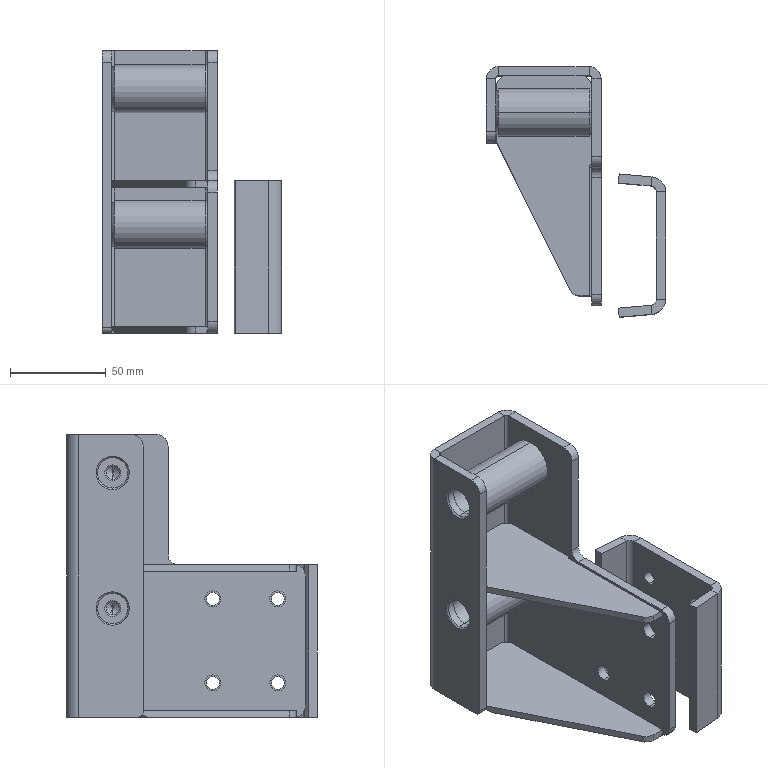Part | STEP file | Symmetry UPPER ROLLER BASE_COUNTER PLATE BASE | 6 solids | 135 faces | box 93.76 x 131.085 x 148 mm | volume 235886 mm3 | plane 66 | cylinder 49 | cone 20 | commonest cylinder face diameters 6.8 x12 8.4 x8 16 x8 12 x6 25 x4 6 x3